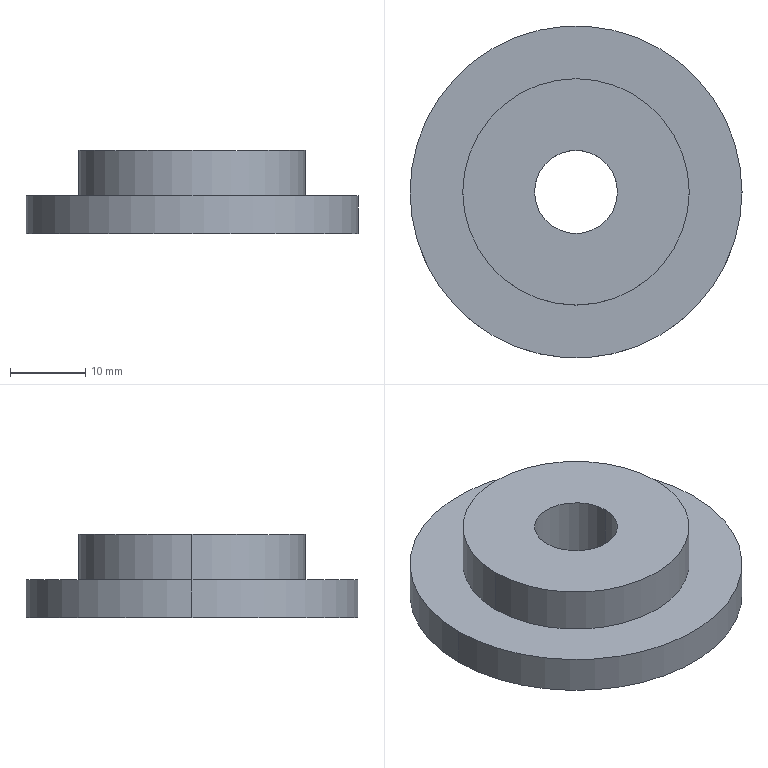Part | SolidWorks | features Revolution 1 | 1 solid | 11 faces | box 44 x 44 x 11 mm | volume 10654 mm3 | cylinder 6 | plane 3 | cone 2 | commonest cylinder face diameters 11 x2 30 x2 44 x2
STEP:
#1=CARTESIAN_POINT('',(22.,0.,-11.));
#2=VERTEX_POINT('',#1);
#3=CARTESIAN_POINT('',(-22.,0.,-11.));
#4=VERTEX_POINT('',#3);
#5=CARTESIAN_POINT('',(0.,0.,-11.));
#6=DIRECTION('',(0.,0.,1.));
#7=DIRECTION('',(1.,0.,0.));
#8=AXIS2_PLACEMENT_3D('',#5,#6,#7);
#9=CIRCLE('',#8,22.);
#10=EDGE_CURVE('',#2,#4,#9,.T.);
#11=ORIENTED_EDGE('',*,*,#10,.T.);
#12=CARTESIAN_POINT('',(-22.,0.,-6.));
#13=VERTEX_POINT('',#12);
#14=CARTESIAN_POINT('',(-22.,0.,17.908));
#15=DIRECTION('',(0.,0.,1.));
#16=VECTOR('',#15,1000.);
#17=LINE('',#14,#16);
#18=EDGE_CURVE('',#4,#13,#17,.T.);
#19=ORIENTED_EDGE('',*,*,#18,.T.);
#20=CARTESIAN_POINT('',(22.,0.,-6.));
#21=VERTEX_POINT('',#20);
#22=CARTESIAN_POINT('',(0.,0.,-6.));
#23=DIRECTION('',(0.,0.,1.));
#24=DIRECTION('',(1.,0.,0.));
#25=AXIS2_PLACEMENT_3D('',#22,#23,#24);
#26=CIRCLE('',#25,22.);
#27=EDGE_CURVE('',#21,#13,#26,.T.);
#28=ORIENTED_EDGE('',*,*,#27,.F.);
#29=CARTESIAN_POINT('',(22.,0.,17.908));
#30=DIRECTION('',(0.,0.,1.));
#31=VECTOR('',#30,1000.);
#32=LINE('',#29,#31);
#33=EDGE_CURVE('',#2,#21,#32,.T.);
#34=ORIENTED_EDGE('',*,*,#33,.F.);
#35=EDGE_LOOP('',(#11,#19,#28,#34));
#36=FACE_OUTER_BOUND('',#35,.T.);
#37=CARTESIAN_POINT('',(0.,0.,17.908));
#38=DIRECTION('',(0.,0.,1.));
#39=DIRECTION('',(1.,0.,0.));
#40=AXIS2_PLACEMENT_3D('',#37,#38,#39);
#41=CYLINDRICAL_SURFACE('',#40,22.);
#42=ADVANCED_FACE('',(#36),#41,.T.);
#43=CARTESIAN_POINT('',(-5.5,0.,-9.));
#44=VERTEX_POINT('',#43);
#45=CARTESIAN_POINT('',(5.5,0.,-9.));
#46=VERTEX_POINT('',#45);
#47=CARTESIAN_POINT('',(0.,0.,-9.));
#48=DIRECTION('',(0.,0.,1.));
#49=DIRECTION('',(1.,0.,0.));
#50=AXIS2_PLACEMENT_3D('',#47,#48,#49);
#51=CIRCLE('',#50,5.5);
#52=EDGE_CURVE('',#44,#46,#51,.T.);
#53=ORIENTED_EDGE('',*,*,#52,.T.);
#54=CARTESIAN_POINT('',(8.964,0.,-11.));
#55=VERTEX_POINT('',#54);
#56=CARTESIAN_POINT('',(5.5,0.,-9.));
#57=DIRECTION('',(0.866,0.,-0.5));
#58=VECTOR('',#57,1000.);
#59=LINE('',#56,#58);
#60=EDGE_CURVE('',#46,#55,#59,.T.);
#61=ORIENTED_EDGE('',*,*,#60,.T.);
#62=CARTESIAN_POINT('',(-8.964,0.,-11.));
#63=VERTEX_POINT('',#62);
#64=CARTESIAN_POINT('',(0.,0.,-11.));
#65=DIRECTION('',(0.,0.,1.));
#66=DIRECTION('',(1.,0.,0.));
#67=AXIS2_PLACEMENT_3D('',#64,#65,#66);
#68=CIRCLE('',#67,8.964);
#69=EDGE_CURVE('',#63,#55,#68,.T.);
#70=ORIENTED_EDGE('',*,*,#69,.F.);
#71=CARTESIAN_POINT('',(-5.5,0.,-9.));
#72=DIRECTION('',(-0.866,0.,-0.5));
#73=VECTOR('',#72,1000.);
#74=LINE('',#71,#73);
#75=EDGE_CURVE('',#44,#63,#74,.T.);
#76=ORIENTED_EDGE('',*,*,#75,.F.);
#77=EDGE_LOOP('',(#53,#61,#70,#76));
#78=FACE_OUTER_BOUND('',#77,.T.);
#79=CARTESIAN_POINT('',(0.,0.,-9.));
#80=DIRECTION('',(0.,0.,-1.));
#81=DIRECTION('',(-1.,0.,0.));
#82=AXIS2_PLACEMENT_3D('',#79,#80,#81);
#83=CONICAL_SURFACE('',#82,5.5,1.047);
#84=ADVANCED_FACE('',(#78),#83,.F.);
#85=ORIENTED_EDGE('',*,*,#52,.F.);
#86=CARTESIAN_POINT('',(-5.5,0.,0.));
#87=VERTEX_POINT('',#86);
#88=CARTESIAN_POINT('',(-5.5,0.,17.908));
#89=DIRECTION('',(0.,0.,1.));
#90=VECTOR('',#89,1000.);
#91=LINE('',#88,#90);
#92=EDGE_CURVE('',#44,#87,#91,.T.);
#93=ORIENTED_EDGE('',*,*,#92,.T.);
#94=CARTESIAN_POINT('',(5.5,0.,0.));
#95=VERTEX_POINT('',#94);
#96=CARTESIAN_POINT('',(0.,0.,0.));
#97=DIRECTION('',(0.,0.,1.));
#98=DIRECTION('',(1.,0.,0.));
#99=AXIS2_PLACEMENT_3D('',#96,#97,#98);
#100=CIRCLE('',#99,5.5);
#101=EDGE_CURVE('',#87,#95,#100,.T.);
#102=ORIENTED_EDGE('',*,*,#101,.T.);
#103=CARTESIAN_POINT('',(5.5,0.,17.908));
#104=DIRECTION('',(0.,0.,1.));
#105=VECTOR('',#104,1000.);
#106=LINE('',#103,#105);
#107=EDGE_CURVE('',#46,#95,#106,.T.);
#108=ORIENTED_EDGE('',*,*,#107,.F.);
#109=EDGE_LOOP('',(#85,#93,#102,#108));
#110=FACE_OUTER_BOUND('',#109,.T.);
#111=CARTESIAN_POINT('',(0.,0.,17.908));
#112=DIRECTION('',(0.,0.,1.));
#113=DIRECTION('',(1.,0.,0.));
#114=AXIS2_PLACEMENT_3D('',#111,#112,#113);
#115=CYLINDRICAL_SURFACE('',#114,5.5);
#116=ADVANCED_FACE('',(#110),#115,.F.);
#117=CARTESIAN_POINT('',(15.,0.,-6.));
#118=VERTEX_POINT('',#117);
#119=CARTESIAN_POINT('',(-15.,0.,-6.));
#120=VERTEX_POINT('',#119);
#121=CARTESIAN_POINT('',(0.,0.,-6.));
#122=DIRECTION('',(0.,0.,1.));
#123=DIRECTION('',(1.,0.,0.));
#124=AXIS2_PLACEMENT_3D('',#121,#122,#123);
#125=CIRCLE('',#124,15.);
#126=EDGE_CURVE('',#118,#120,#125,.T.);
#127=ORIENTED_EDGE('',*,*,#126,.T.);
#128=CARTESIAN_POINT('',(-15.,0.,0.));
#129=VERTEX_POINT('',#128);
#130=CARTESIAN_POINT('',(-15.,0.,17.908));
#131=DIRECTION('',(0.,0.,1.));
#132=VECTOR('',#131,1000.);
#133=LINE('',#130,#132);
#134=EDGE_CURVE('',#120,#129,#133,.T.);
#135=ORIENTED_EDGE('',*,*,#134,.T.);
#136=CARTESIAN_POINT('',(15.,0.,0.));
#137=VERTEX_POINT('',#136);
#138=CARTESIAN_POINT('',(0.,0.,0.));
#139=DIRECTION('',(0.,0.,1.));
#140=DIRECTION('',(1.,0.,0.));
#141=AXIS2_PLACEMENT_3D('',#138,#139,#140);
#142=CIRCLE('',#141,15.);
#143=EDGE_CURVE('',#137,#129,#142,.T.);
#144=ORIENTED_EDGE('',*,*,#143,.F.);
#145=CARTESIAN_POINT('',(15.,0.,17.908));
#146=DIRECTION('',(0.,0.,1.));
#147=VECTOR('',#146,1000.);
#148=LINE('',#145,#147);
#149=EDGE_CURVE('',#118,#137,#148,.T.);
#150=ORIENTED_EDGE('',*,*,#149,.F.);
#151=EDGE_LOOP('',(#127,#135,#144,#150));
#152=FACE_OUTER_BOUND('',#151,.T.);
#153=CARTESIAN_POINT('',(0.,0.,17.908));
#154=DIRECTION('',(0.,0.,1.));
#155=DIRECTION('',(1.,0.,0.));
#156=AXIS2_PLACEMENT_3D('',#153,#154,#155);
#157=CYLINDRICAL_SURFACE('',#156,15.);
#158=ADVANCED_FACE('',(#152),#157,.T.);
#159=ORIENTED_EDGE('',*,*,#134,.F.);
#160=CARTESIAN_POINT('',(0.,0.,-6.));
#161=DIRECTION('',(0.,0.,1.));
#162=DIRECTION('',(1.,0.,0.));
#163=AXIS2_PLACEMENT_3D('',#160,#161,#162);
#164=CIRCLE('',#163,15.);
#165=EDGE_CURVE('',#120,#118,#164,.T.);
#166=ORIENTED_EDGE('',*,*,#165,.T.);
#167=ORIENTED_EDGE('',*,*,#149,.T.);
#168=CARTESIAN_POINT('',(0.,0.,0.));
#169=DIRECTION('',(0.,0.,1.));
#170=DIRECTION('',(1.,0.,0.));
#171=AXIS2_PLACEMENT_3D('',#168,#169,#170);
#172=CIRCLE('',#171,15.);
#173=EDGE_CURVE('',#129,#137,#172,.T.);
#174=ORIENTED_EDGE('',*,*,#173,.F.);
#175=EDGE_LOOP('',(#159,#166,#167,#174));
#176=FACE_OUTER_BOUND('',#175,.T.);
#177=CARTESIAN_POINT('',(0.,0.,17.908));
#178=DIRECTION('',(0.,0.,1.));
#179=DIRECTION('',(1.,0.,0.));
#180=AXIS2_PLACEMENT_3D('',#177,#178,#179);
#181=CYLINDRICAL_SURFACE('',#180,15.);
#182=ADVANCED_FACE('',(#176),#181,.T.);
#183=CARTESIAN_POINT('',(0.,0.,0.));
#184=DIRECTION('',(0.,0.,1.));
#185=DIRECTION('',(1.,0.,0.));
#186=AXIS2_PLACEMENT_3D('',#183,#184,#185);
#187=CIRCLE('',#186,5.5);
#188=EDGE_CURVE('',#95,#87,#187,.T.);
#189=ORIENTED_EDGE('',*,*,#188,.F.);
#190=ORIENTED_EDGE('',*,*,#101,.F.);
#191=EDGE_LOOP('',(#189,#190));
#192=FACE_BOUND('',#191,.T.);
#193=ORIENTED_EDGE('',*,*,#143,.T.);
#194=ORIENTED_EDGE('',*,*,#173,.T.);
#195=EDGE_LOOP('',(#193,#194));
#196=FACE_OUTER_BOUND('',#195,.T.);
#197=CARTESIAN_POINT('',(0.,15.,0.));
#198=DIRECTION('',(0.,0.,-1.));
#199=DIRECTION('',(-1.,0.,0.));
#200=AXIS2_PLACEMENT_3D('',#197,#198,#199);
#201=PLANE('',#200);
#202=ADVANCED_FACE('',(#192,#196),#201,.F.);
#203=ORIENTED_EDGE('',*,*,#92,.F.);
#204=CARTESIAN_POINT('',(0.,0.,-9.));
#205=DIRECTION('',(0.,0.,1.));
#206=DIRECTION('',(1.,0.,0.));
#207=AXIS2_PLACEMENT_3D('',#204,#205,#206);
#208=CIRCLE('',#207,5.5);
#209=EDGE_CURVE('',#46,#44,#208,.T.);
#210=ORIENTED_EDGE('',*,*,#209,.F.);
#211=ORIENTED_EDGE('',*,*,#107,.T.);
#212=ORIENTED_EDGE('',*,*,#188,.T.);
#213=EDGE_LOOP('',(#203,#210,#211,#212));
#214=FACE_OUTER_BOUND('',#213,.T.);
#215=CARTESIAN_POINT('',(0.,0.,17.908));
#216=DIRECTION('',(0.,0.,1.));
#217=DIRECTION('',(1.,0.,0.));
#218=AXIS2_PLACEMENT_3D('',#215,#216,#217);
#219=CYLINDRICAL_SURFACE('',#218,5.5);
#220=ADVANCED_FACE('',(#214),#219,.F.);
#221=ORIENTED_EDGE('',*,*,#60,.F.);
#222=ORIENTED_EDGE('',*,*,#209,.T.);
#223=ORIENTED_EDGE('',*,*,#75,.T.);
#224=CARTESIAN_POINT('',(0.,0.,-11.));
#225=DIRECTION('',(0.,0.,1.));
#226=DIRECTION('',(1.,0.,0.));
#227=AXIS2_PLACEMENT_3D('',#224,#225,#226);
#228=CIRCLE('',#227,8.964);
#229=EDGE_CURVE('',#55,#63,#228,.T.);
#230=ORIENTED_EDGE('',*,*,#229,.F.);
#231=EDGE_LOOP('',(#221,#222,#223,#230));
#232=FACE_OUTER_BOUND('',#231,.T.);
#233=CARTESIAN_POINT('',(0.,0.,-9.));
#234=DIRECTION('',(0.,0.,-1.));
#235=DIRECTION('',(-1.,0.,0.));
#236=AXIS2_PLACEMENT_3D('',#233,#234,#235);
#237=CONICAL_SURFACE('',#236,5.5,1.047);
#238=ADVANCED_FACE('',(#232),#237,.F.);
#239=ORIENTED_EDGE('',*,*,#10,.F.);
#240=CARTESIAN_POINT('',(0.,0.,-11.));
#241=DIRECTION('',(0.,0.,1.));
#242=DIRECTION('',(1.,0.,0.));
#243=AXIS2_PLACEMENT_3D('',#240,#241,#242);
#244=CIRCLE('',#243,22.);
#245=EDGE_CURVE('',#4,#2,#244,.T.);
#246=ORIENTED_EDGE('',*,*,#245,.F.);
#247=EDGE_LOOP('',(#239,#246));
#248=FACE_OUTER_BOUND('',#247,.T.);
#249=ORIENTED_EDGE('',*,*,#69,.T.);
#250=ORIENTED_EDGE('',*,*,#229,.T.);
#251=EDGE_LOOP('',(#249,#250));
#252=FACE_BOUND('',#251,.T.);
#253=CARTESIAN_POINT('',(0.,8.964,-11.));
#254=DIRECTION('',(0.,0.,1.));
#255=DIRECTION('',(1.,0.,0.));
#256=AXIS2_PLACEMENT_3D('',#253,#254,#255);
#257=PLANE('',#256);
#258=ADVANCED_FACE('',(#248,#252),#257,.F.);
#259=ORIENTED_EDGE('',*,*,#18,.F.);
#260=ORIENTED_EDGE('',*,*,#245,.T.);
#261=ORIENTED_EDGE('',*,*,#33,.T.);
#262=CARTESIAN_POINT('',(0.,0.,-6.));
#263=DIRECTION('',(0.,0.,1.));
#264=DIRECTION('',(1.,0.,0.));
#265=AXIS2_PLACEMENT_3D('',#262,#263,#264);
#266=CIRCLE('',#265,22.);
#267=EDGE_CURVE('',#13,#21,#266,.T.);
#268=ORIENTED_EDGE('',*,*,#267,.F.);
#269=EDGE_LOOP('',(#259,#260,#261,#268));
#270=FACE_OUTER_BOUND('',#269,.T.);
#271=CARTESIAN_POINT('',(0.,0.,17.908));
#272=DIRECTION('',(0.,0.,1.));
#273=DIRECTION('',(1.,0.,0.));
#274=AXIS2_PLACEMENT_3D('',#271,#272,#273);
#275=CYLINDRICAL_SURFACE('',#274,22.);
#276=ADVANCED_FACE('',(#270),#275,.T.);
#277=ORIENTED_EDGE('',*,*,#126,.F.);
#278=ORIENTED_EDGE('',*,*,#165,.F.);
#279=EDGE_LOOP('',(#277,#278));
#280=FACE_BOUND('',#279,.T.);
#281=ORIENTED_EDGE('',*,*,#27,.T.);
#282=ORIENTED_EDGE('',*,*,#267,.T.);
#283=EDGE_LOOP('',(#281,#282));
#284=FACE_OUTER_BOUND('',#283,.T.);
#285=CARTESIAN_POINT('',(0.,22.,-6.));
#286=DIRECTION('',(0.,0.,-1.));
#287=DIRECTION('',(-1.,0.,0.));
#288=AXIS2_PLACEMENT_3D('',#285,#286,#287);
#289=PLANE('',#288);
#290=ADVANCED_FACE('',(#280,#284),#289,.F.);
#291=CLOSED_SHELL('',(#42,#84,#116,#158,#182,#202,#220,#238,#258,#276,#290));
#292=MANIFOLD_SOLID_BREP('',#291);
#293=CARTESIAN_POINT('',(0.,0.,0.));
#294=DIRECTION('',(0.,0.,1.));
#295=DIRECTION('',(1.,0.,0.));
#296=AXIS2_PLACEMENT_3D('',#293,#294,#295);
#297=(LENGTH_UNIT()NAMED_UNIT(*)SI_UNIT(.MILLI.,.METRE.));
#298=UNCERTAINTY_MEASURE_WITH_UNIT(LENGTH_MEASURE(0.00001),#297,'','');
#299=(NAMED_UNIT(*)PLANE_ANGLE_UNIT()SI_UNIT($,.RADIAN.));
#300=(NAMED_UNIT(*)SI_UNIT($,.STERADIAN.)SOLID_ANGLE_UNIT());
#301=(GEOMETRIC_REPRESENTATION_CONTEXT(3)GLOBAL_UNCERTAINTY_ASSIGNED_CONTEXT((#298))GLOBAL_UNIT_ASSIGNED_CONTEXT((#297,#299,#300))REPRESENTATION_CONTEXT('',''));
#302=ADVANCED_BREP_SHAPE_REPRESENTATION('',(#292,#296),#301);